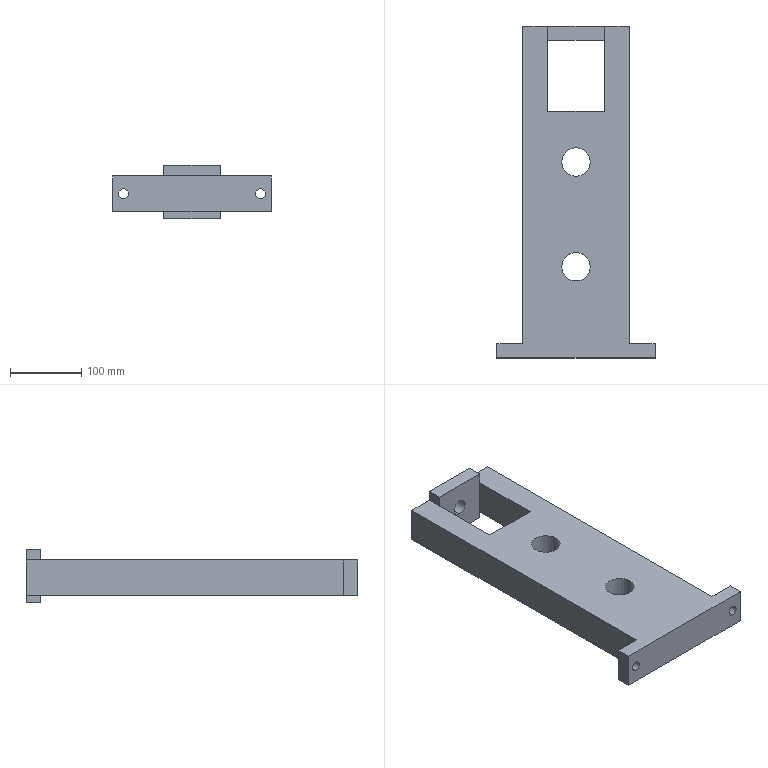Part | SolidWorks | features BaseBody 2 | 2 solids | 30 faces | box 222 x 466.001 x 75 mm | volume 3067581 mm3 | plane 20 | cylinder 10 | commonest cylinder face diameters 14 x4 40 x4 22 x2
STEP:
#1=CARTESIAN_POINT('',(0.,436.001,-8.5));
#2=VERTEX_POINT('',#1);
#3=CARTESIAN_POINT('',(0.,436.001,13.5));
#4=VERTEX_POINT('',#3);
#5=CARTESIAN_POINT('',(0.,436.001,2.5));
#6=DIRECTION('',(0.,1.,0.));
#7=DIRECTION('',(0.,0.,1.));
#8=AXIS2_PLACEMENT_3D('',#5,#6,#7);
#9=CIRCLE('',#8,11.);
#10=EDGE_CURVE('',#2,#4,#9,.T.);
#11=ORIENTED_EDGE('',*,*,#10,.F.);
#12=CARTESIAN_POINT('',(0.,456.001,-8.5));
#13=VERTEX_POINT('',#12);
#14=CARTESIAN_POINT('',(0.,456.001,-8.5));
#15=DIRECTION('',(0.,1.,0.));
#16=VECTOR('',#15,1000.);
#17=LINE('',#14,#16);
#18=EDGE_CURVE('',#2,#13,#17,.T.);
#19=ORIENTED_EDGE('',*,*,#18,.T.);
#20=CARTESIAN_POINT('',(0.,456.001,13.5));
#21=VERTEX_POINT('',#20);
#22=CARTESIAN_POINT('',(0.,456.001,2.5));
#23=DIRECTION('',(0.,1.,0.));
#24=DIRECTION('',(0.,0.,1.));
#25=AXIS2_PLACEMENT_3D('',#22,#23,#24);
#26=CIRCLE('',#25,11.);
#27=EDGE_CURVE('',#13,#21,#26,.T.);
#28=ORIENTED_EDGE('',*,*,#27,.T.);
#29=CARTESIAN_POINT('',(0.,456.001,13.5));
#30=DIRECTION('',(0.,1.,0.));
#31=VECTOR('',#30,1000.);
#32=LINE('',#29,#31);
#33=EDGE_CURVE('',#4,#21,#32,.T.);
#34=ORIENTED_EDGE('',*,*,#33,.F.);
#35=EDGE_LOOP('',(#11,#19,#28,#34));
#36=FACE_OUTER_BOUND('',#35,.T.);
#37=CARTESIAN_POINT('',(0.,456.001,2.5));
#38=DIRECTION('',(0.,1.,0.));
#39=DIRECTION('',(0.,0.,1.));
#40=AXIS2_PLACEMENT_3D('',#37,#38,#39);
#41=CYLINDRICAL_SURFACE('',#40,11.);
#42=ADVANCED_FACE('',(#36),#41,.F.);
#43=CARTESIAN_POINT('',(-40.,456.001,-35.));
#44=VERTEX_POINT('',#43);
#45=CARTESIAN_POINT('',(-40.,436.001,-35.));
#46=VERTEX_POINT('',#45);
#47=CARTESIAN_POINT('',(-40.,456.001,-35.));
#48=DIRECTION('',(0.,-1.,0.));
#49=VECTOR('',#48,1000.);
#50=LINE('',#47,#49);
#51=EDGE_CURVE('',#44,#46,#50,.T.);
#52=ORIENTED_EDGE('',*,*,#51,.F.);
#53=CARTESIAN_POINT('',(40.,456.001,-35.));
#54=VERTEX_POINT('',#53);
#55=CARTESIAN_POINT('',(-40.,456.001,-35.));
#56=DIRECTION('',(-1.,0.,0.));
#57=VECTOR('',#56,1000.);
#58=LINE('',#55,#57);
#59=EDGE_CURVE('',#54,#44,#58,.T.);
#60=ORIENTED_EDGE('',*,*,#59,.F.);
#61=CARTESIAN_POINT('',(40.,436.001,-35.));
#62=VERTEX_POINT('',#61);
#63=CARTESIAN_POINT('',(40.,456.001,-35.));
#64=DIRECTION('',(0.,1.,0.));
#65=VECTOR('',#64,1000.);
#66=LINE('',#63,#65);
#67=EDGE_CURVE('',#62,#54,#66,.T.);
#68=ORIENTED_EDGE('',*,*,#67,.F.);
#69=CARTESIAN_POINT('',(-40.,436.001,-35.));
#70=DIRECTION('',(1.,0.,0.));
#71=VECTOR('',#70,1000.);
#72=LINE('',#69,#71);
#73=EDGE_CURVE('',#46,#62,#72,.T.);
#74=ORIENTED_EDGE('',*,*,#73,.F.);
#75=EDGE_LOOP('',(#52,#60,#68,#74));
#76=FACE_OUTER_BOUND('',#75,.T.);
#77=CARTESIAN_POINT('',(0.,0.,-35.));
#78=DIRECTION('',(0.,0.,1.));
#79=DIRECTION('',(1.,0.,0.));
#80=AXIS2_PLACEMENT_3D('',#77,#78,#79);
#81=PLANE('',#80);
#82=ADVANCED_FACE('',(#76),#81,.F.);
#83=CARTESIAN_POINT('',(-40.,456.001,40.));
#84=VERTEX_POINT('',#83);
#85=CARTESIAN_POINT('',(-40.,436.001,40.));
#86=VERTEX_POINT('',#85);
#87=CARTESIAN_POINT('',(-40.,456.001,40.));
#88=DIRECTION('',(0.,-1.,0.));
#89=VECTOR('',#88,1000.);
#90=LINE('',#87,#89);
#91=EDGE_CURVE('',#84,#86,#90,.T.);
#92=ORIENTED_EDGE('',*,*,#91,.T.);
#93=CARTESIAN_POINT('',(40.,436.001,40.));
#94=VERTEX_POINT('',#93);
#95=CARTESIAN_POINT('',(-40.,436.001,40.));
#96=DIRECTION('',(1.,0.,0.));
#97=VECTOR('',#96,1000.);
#98=LINE('',#95,#97);
#99=EDGE_CURVE('',#86,#94,#98,.T.);
#100=ORIENTED_EDGE('',*,*,#99,.T.);
#101=CARTESIAN_POINT('',(40.,456.001,40.));
#102=VERTEX_POINT('',#101);
#103=CARTESIAN_POINT('',(40.,456.001,40.));
#104=DIRECTION('',(0.,1.,0.));
#105=VECTOR('',#104,1000.);
#106=LINE('',#103,#105);
#107=EDGE_CURVE('',#94,#102,#106,.T.);
#108=ORIENTED_EDGE('',*,*,#107,.T.);
#109=CARTESIAN_POINT('',(-40.,456.001,40.));
#110=DIRECTION('',(-1.,0.,0.));
#111=VECTOR('',#110,1000.);
#112=LINE('',#109,#111);
#113=EDGE_CURVE('',#102,#84,#112,.T.);
#114=ORIENTED_EDGE('',*,*,#113,.T.);
#115=EDGE_LOOP('',(#92,#100,#108,#114));
#116=FACE_OUTER_BOUND('',#115,.T.);
#117=CARTESIAN_POINT('',(0.,0.,40.));
#118=DIRECTION('',(0.,0.,1.));
#119=DIRECTION('',(1.,0.,0.));
#120=AXIS2_PLACEMENT_3D('',#117,#118,#119);
#121=PLANE('',#120);
#122=ADVANCED_FACE('',(#116),#121,.T.);
#123=CARTESIAN_POINT('',(0.,456.001,2.5));
#124=DIRECTION('',(0.,1.,0.));
#125=DIRECTION('',(0.,0.,1.));
#126=AXIS2_PLACEMENT_3D('',#123,#124,#125);
#127=CIRCLE('',#126,11.);
#128=EDGE_CURVE('',#21,#13,#127,.T.);
#129=ORIENTED_EDGE('',*,*,#128,.F.);
#130=ORIENTED_EDGE('',*,*,#27,.F.);
#131=EDGE_LOOP('',(#129,#130));
#132=FACE_BOUND('',#131,.T.);
#133=ORIENTED_EDGE('',*,*,#59,.T.);
#134=CARTESIAN_POINT('',(-40.,456.001,40.));
#135=DIRECTION('',(0.,0.,-1.));
#136=VECTOR('',#135,1000.);
#137=LINE('',#134,#136);
#138=EDGE_CURVE('',#84,#44,#137,.T.);
#139=ORIENTED_EDGE('',*,*,#138,.F.);
#140=ORIENTED_EDGE('',*,*,#113,.F.);
#141=CARTESIAN_POINT('',(40.,456.001,40.));
#142=DIRECTION('',(0.,0.,-1.));
#143=VECTOR('',#142,1000.);
#144=LINE('',#141,#143);
#145=EDGE_CURVE('',#102,#54,#144,.T.);
#146=ORIENTED_EDGE('',*,*,#145,.T.);
#147=EDGE_LOOP('',(#133,#139,#140,#146));
#148=FACE_OUTER_BOUND('',#147,.T.);
#149=CARTESIAN_POINT('',(-40.,456.001,40.));
#150=DIRECTION('',(0.,-1.,0.));
#151=DIRECTION('',(0.,0.,-1.));
#152=AXIS2_PLACEMENT_3D('',#149,#150,#151);
#153=PLANE('',#152);
#154=ADVANCED_FACE('',(#132,#148),#153,.F.);
#155=ORIENTED_EDGE('',*,*,#67,.T.);
#156=ORIENTED_EDGE('',*,*,#145,.F.);
#157=ORIENTED_EDGE('',*,*,#107,.F.);
#158=CARTESIAN_POINT('',(40.,436.001,40.));
#159=DIRECTION('',(0.,0.,-1.));
#160=VECTOR('',#159,1000.);
#161=LINE('',#158,#160);
#162=EDGE_CURVE('',#94,#62,#161,.T.);
#163=ORIENTED_EDGE('',*,*,#162,.T.);
#164=EDGE_LOOP('',(#155,#156,#157,#163));
#165=FACE_OUTER_BOUND('',#164,.T.);
#166=CARTESIAN_POINT('',(40.,456.001,40.));
#167=DIRECTION('',(-1.,0.,0.));
#168=DIRECTION('',(0.,0.,1.));
#169=AXIS2_PLACEMENT_3D('',#166,#167,#168);
#170=PLANE('',#169);
#171=ADVANCED_FACE('',(#165),#170,.F.);
#172=CARTESIAN_POINT('',(0.,436.001,2.5));
#173=DIRECTION('',(0.,1.,0.));
#174=DIRECTION('',(0.,0.,1.));
#175=AXIS2_PLACEMENT_3D('',#172,#173,#174);
#176=CIRCLE('',#175,11.);
#177=EDGE_CURVE('',#4,#2,#176,.T.);
#178=ORIENTED_EDGE('',*,*,#177,.T.);
#179=ORIENTED_EDGE('',*,*,#10,.T.);
#180=EDGE_LOOP('',(#178,#179));
#181=FACE_BOUND('',#180,.T.);
#182=ORIENTED_EDGE('',*,*,#73,.T.);
#183=ORIENTED_EDGE('',*,*,#162,.F.);
#184=ORIENTED_EDGE('',*,*,#99,.F.);
#185=CARTESIAN_POINT('',(-40.,436.001,40.));
#186=DIRECTION('',(0.,0.,-1.));
#187=VECTOR('',#186,1000.);
#188=LINE('',#185,#187);
#189=EDGE_CURVE('',#86,#46,#188,.T.);
#190=ORIENTED_EDGE('',*,*,#189,.T.);
#191=EDGE_LOOP('',(#182,#183,#184,#190));
#192=FACE_OUTER_BOUND('',#191,.T.);
#193=CARTESIAN_POINT('',(-40.,436.001,40.));
#194=DIRECTION('',(0.,1.,0.));
#195=DIRECTION('',(1.,0.,0.));
#196=AXIS2_PLACEMENT_3D('',#193,#194,#195);
#197=PLANE('',#196);
#198=ADVANCED_FACE('',(#181,#192),#197,.F.);
#199=ORIENTED_EDGE('',*,*,#51,.T.);
#200=ORIENTED_EDGE('',*,*,#189,.F.);
#201=ORIENTED_EDGE('',*,*,#91,.F.);
#202=ORIENTED_EDGE('',*,*,#138,.T.);
#203=EDGE_LOOP('',(#199,#200,#201,#202));
#204=FACE_OUTER_BOUND('',#203,.T.);
#205=CARTESIAN_POINT('',(-40.,456.001,40.));
#206=DIRECTION('',(1.,0.,0.));
#207=DIRECTION('',(0.,1.,0.));
#208=AXIS2_PLACEMENT_3D('',#205,#206,#207);
#209=PLANE('',#208);
#210=ADVANCED_FACE('',(#204),#209,.F.);
#211=ORIENTED_EDGE('',*,*,#18,.F.);
#212=ORIENTED_EDGE('',*,*,#177,.F.);
#213=ORIENTED_EDGE('',*,*,#33,.T.);
#214=ORIENTED_EDGE('',*,*,#128,.T.);
#215=EDGE_LOOP('',(#211,#212,#213,#214));
#216=FACE_OUTER_BOUND('',#215,.T.);
#217=CARTESIAN_POINT('',(0.,456.001,2.5));
#218=DIRECTION('',(0.,1.,0.));
#219=DIRECTION('',(0.,0.,1.));
#220=AXIS2_PLACEMENT_3D('',#217,#218,#219);
#221=CYLINDRICAL_SURFACE('',#220,11.);
#222=ADVANCED_FACE('',(#216),#221,.F.);
#223=CLOSED_SHELL('',(#42,#82,#122,#154,#171,#198,#210,#222));
#224=MANIFOLD_SOLID_BREP('',#223);
#225=CARTESIAN_POINT('',(-96.,-10.,-7.));
#226=VERTEX_POINT('',#225);
#227=CARTESIAN_POINT('',(-96.,-10.,7.));
#228=VERTEX_POINT('',#227);
#229=CARTESIAN_POINT('',(-96.,-10.,0.));
#230=DIRECTION('',(0.,1.,0.));
#231=DIRECTION('',(-1.,0.,0.));
#232=AXIS2_PLACEMENT_3D('',#229,#230,#231);
#233=CIRCLE('',#232,7.);
#234=EDGE_CURVE('',#226,#228,#233,.T.);
#235=ORIENTED_EDGE('',*,*,#234,.F.);
#236=CARTESIAN_POINT('',(-96.,10.,-7.));
#237=VERTEX_POINT('',#236);
#238=CARTESIAN_POINT('',(-96.,10.,-7.));
#239=DIRECTION('',(0.,1.,0.));
#240=VECTOR('',#239,1000.);
#241=LINE('',#238,#240);
#242=EDGE_CURVE('',#226,#237,#241,.T.);
#243=ORIENTED_EDGE('',*,*,#242,.T.);
#244=CARTESIAN_POINT('',(-96.,10.,7.));
#245=VERTEX_POINT('',#244);
#246=CARTESIAN_POINT('',(-96.,10.,0.));
#247=DIRECTION('',(0.,1.,0.));
#248=DIRECTION('',(1.,0.,0.));
#249=AXIS2_PLACEMENT_3D('',#246,#247,#248);
#250=CIRCLE('',#249,7.);
#251=EDGE_CURVE('',#237,#245,#250,.T.);
#252=ORIENTED_EDGE('',*,*,#251,.T.);
#253=CARTESIAN_POINT('',(-96.,10.,7.));
#254=DIRECTION('',(0.,1.,0.));
#255=VECTOR('',#254,1000.);
#256=LINE('',#253,#255);
#257=EDGE_CURVE('',#228,#245,#256,.T.);
#258=ORIENTED_EDGE('',*,*,#257,.F.);
#259=EDGE_LOOP('',(#235,#243,#252,#258));
#260=FACE_OUTER_BOUND('',#259,.T.);
#261=CARTESIAN_POINT('',(-96.,10.,0.));
#262=DIRECTION('',(0.,1.,0.));
#263=DIRECTION('',(0.,0.,1.));
#264=AXIS2_PLACEMENT_3D('',#261,#262,#263);
#265=CYLINDRICAL_SURFACE('',#264,7.);
#266=ADVANCED_FACE('',(#260),#265,.F.);
#267=CARTESIAN_POINT('',(96.,-10.,-7.));
#268=VERTEX_POINT('',#267);
#269=CARTESIAN_POINT('',(96.,-10.,7.));
#270=VERTEX_POINT('',#269);
#271=CARTESIAN_POINT('',(96.,-10.,0.));
#272=DIRECTION('',(0.,1.,0.));
#273=DIRECTION('',(-1.,0.,0.));
#274=AXIS2_PLACEMENT_3D('',#271,#272,#273);
#275=CIRCLE('',#274,7.);
#276=EDGE_CURVE('',#268,#270,#275,.T.);
#277=ORIENTED_EDGE('',*,*,#276,.F.);
#278=CARTESIAN_POINT('',(96.,10.,-7.));
#279=VERTEX_POINT('',#278);
#280=CARTESIAN_POINT('',(96.,10.,-7.));
#281=DIRECTION('',(0.,1.,0.));
#282=VECTOR('',#281,1000.);
#283=LINE('',#280,#282);
#284=EDGE_CURVE('',#268,#279,#283,.T.);
#285=ORIENTED_EDGE('',*,*,#284,.T.);
#286=CARTESIAN_POINT('',(96.,10.,7.));
#287=VERTEX_POINT('',#286);
#288=CARTESIAN_POINT('',(96.,10.,0.));
#289=DIRECTION('',(0.,1.,0.));
#290=DIRECTION('',(1.,0.,0.));
#291=AXIS2_PLACEMENT_3D('',#288,#289,#290);
#292=CIRCLE('',#291,7.);
#293=EDGE_CURVE('',#279,#287,#292,.T.);
#294=ORIENTED_EDGE('',*,*,#293,.T.);
#295=CARTESIAN_POINT('',(96.,10.,7.));
#296=DIRECTION('',(0.,1.,0.));
#297=VECTOR('',#296,1000.);
#298=LINE('',#295,#297);
#299=EDGE_CURVE('',#270,#287,#298,.T.);
#300=ORIENTED_EDGE('',*,*,#299,.F.);
#301=EDGE_LOOP('',(#277,#285,#294,#300));
#302=FACE_OUTER_BOUND('',#301,.T.);
#303=CARTESIAN_POINT('',(96.,10.,0.));
#304=DIRECTION('',(0.,1.,0.));
#305=DIRECTION('',(0.,0.,1.));
#306=AXIS2_PLACEMENT_3D('',#303,#304,#305);
#307=CYLINDRICAL_SURFACE('',#306,7.);
#308=ADVANCED_FACE('',(#302),#307,.F.);
#309=CARTESIAN_POINT('',(-20.,265.,25.));
#310=VERTEX_POINT('',#309);
#311=CARTESIAN_POINT('',(20.,265.,25.));
#312=VERTEX_POINT('',#311);
#313=CARTESIAN_POINT('',(0.,265.,25.));
#314=DIRECTION('',(0.,0.,1.));
#315=DIRECTION('',(1.,0.,0.));
#316=AXIS2_PLACEMENT_3D('',#313,#314,#315);
#317=CIRCLE('',#316,20.);
#318=EDGE_CURVE('',#310,#312,#317,.T.);
#319=ORIENTED_EDGE('',*,*,#318,.T.);
#320=CARTESIAN_POINT('',(20.,265.,-25.));
#321=VERTEX_POINT('',#320);
#322=CARTESIAN_POINT('',(20.,265.,20.));
#323=DIRECTION('',(0.,0.,-1.));
#324=VECTOR('',#323,1000.);
#325=LINE('',#322,#324);
#326=EDGE_CURVE('',#312,#321,#325,.T.);
#327=ORIENTED_EDGE('',*,*,#326,.T.);
#328=CARTESIAN_POINT('',(-20.,265.,-25.));
#329=VERTEX_POINT('',#328);
#330=CARTESIAN_POINT('',(0.,265.,-25.));
#331=DIRECTION('',(0.,0.,1.));
#332=DIRECTION('',(1.,0.,0.));
#333=AXIS2_PLACEMENT_3D('',#330,#331,#332);
#334=CIRCLE('',#333,20.);
#335=EDGE_CURVE('',#329,#321,#334,.T.);
#336=ORIENTED_EDGE('',*,*,#335,.F.);
#337=CARTESIAN_POINT('',(-20.,265.,20.));
#338=DIRECTION('',(0.,0.,-1.));
#339=VECTOR('',#338,1000.);
#340=LINE('',#337,#339);
#341=EDGE_CURVE('',#310,#329,#340,.T.);
#342=ORIENTED_EDGE('',*,*,#341,.F.);
#343=EDGE_LOOP('',(#319,#327,#336,#342));
#344=FACE_OUTER_BOUND('',#343,.T.);
#345=CARTESIAN_POINT('',(0.,265.,20.));
#346=DIRECTION('',(0.,0.,-1.));
#347=DIRECTION('',(-1.,0.,0.));
#348=AXIS2_PLACEMENT_3D('',#345,#346,#347);
#349=CYLINDRICAL_SURFACE('',#348,20.);
#350=ADVANCED_FACE('',(#344),#349,.F.);
#351=CARTESIAN_POINT('',(-20.,118.,25.));
#352=VERTEX_POINT('',#351);
#353=CARTESIAN_POINT('',(20.,118.,25.));
#354=VERTEX_POINT('',#353);
#355=CARTESIAN_POINT('',(0.,118.,25.));
#356=DIRECTION('',(0.,0.,1.));
#357=DIRECTION('',(1.,0.,0.));
#358=AXIS2_PLACEMENT_3D('',#355,#356,#357);
#359=CIRCLE('',#358,20.);
#360=EDGE_CURVE('',#352,#354,#359,.T.);
#361=ORIENTED_EDGE('',*,*,#360,.T.);
#362=CARTESIAN_POINT('',(20.,118.,-25.));
#363=VERTEX_POINT('',#362);
#364=CARTESIAN_POINT('',(20.,118.,20.));
#365=DIRECTION('',(0.,0.,-1.));
#366=VECTOR('',#365,1000.);
#367=LINE('',#364,#366);
#368=EDGE_CURVE('',#354,#363,#367,.T.);
#369=ORIENTED_EDGE('',*,*,#368,.T.);
#370=CARTESIAN_POINT('',(-20.,118.,-25.));
#371=VERTEX_POINT('',#370);
#372=CARTESIAN_POINT('',(0.,118.,-25.));
#373=DIRECTION('',(0.,0.,1.));
#374=DIRECTION('',(1.,0.,0.));
#375=AXIS2_PLACEMENT_3D('',#372,#373,#374);
#376=CIRCLE('',#375,20.);
#377=EDGE_CURVE('',#371,#363,#376,.T.);
#378=ORIENTED_EDGE('',*,*,#377,.F.);
#379=CARTESIAN_POINT('',(-20.,118.,20.));
#380=DIRECTION('',(0.,0.,-1.));
#381=VECTOR('',#380,1000.);
#382=LINE('',#379,#381);
#383=EDGE_CURVE('',#352,#371,#382,.T.);
#384=ORIENTED_EDGE('',*,*,#383,.F.);
#385=EDGE_LOOP('',(#361,#369,#378,#384));
#386=FACE_OUTER_BOUND('',#385,.T.);
#387=CARTESIAN_POINT('',(0.,118.,20.));
#388=DIRECTION('',(0.,0.,-1.));
#389=DIRECTION('',(-1.,0.,0.));
#390=AXIS2_PLACEMENT_3D('',#387,#388,#389);
#391=CYLINDRICAL_SURFACE('',#390,20.);
#392=ADVANCED_FACE('',(#386),#391,.F.);
#393=CARTESIAN_POINT('',(40.,336.001,-25.));
#394=VERTEX_POINT('',#393);
#395=CARTESIAN_POINT('',(-40.,336.001,-25.));
#396=VERTEX_POINT('',#395);
#397=CARTESIAN_POINT('',(-40.,336.001,-25.));
#398=DIRECTION('',(-1.,0.,0.));
#399=VECTOR('',#398,1000.);
#400=LINE('',#397,#399);
#401=EDGE_CURVE('',#394,#396,#400,.T.);
#402=ORIENTED_EDGE('',*,*,#401,.T.);
#403=CARTESIAN_POINT('',(-40.,336.001,25.));
#404=VERTEX_POINT('',#403);
#405=CARTESIAN_POINT('',(-40.,336.001,-25.001));
#406=DIRECTION('',(0.,0.,1.));
#407=VECTOR('',#406,1000.);
#408=LINE('',#405,#407);
#409=EDGE_CURVE('',#396,#404,#408,.T.);
#410=ORIENTED_EDGE('',*,*,#409,.T.);
#411=CARTESIAN_POINT('',(40.,336.001,25.));
#412=VERTEX_POINT('',#411);
#413=CARTESIAN_POINT('',(0.,336.001,25.));
#414=DIRECTION('',(1.,0.,0.));
#415=VECTOR('',#414,1000.);
#416=LINE('',#413,#415);
#417=EDGE_CURVE('',#404,#412,#416,.T.);
#418=ORIENTED_EDGE('',*,*,#417,.T.);
#419=CARTESIAN_POINT('',(40.,336.001,-25.001));
#420=DIRECTION('',(0.,0.,1.));
#421=VECTOR('',#420,1000.);
#422=LINE('',#419,#421);
#423=EDGE_CURVE('',#394,#412,#422,.T.);
#424=ORIENTED_EDGE('',*,*,#423,.F.);
#425=EDGE_LOOP('',(#402,#410,#418,#424));
#426=FACE_OUTER_BOUND('',#425,.T.);
#427=CARTESIAN_POINT('',(-40.,336.001,-25.001));
#428=DIRECTION('',(0.,-1.,0.));
#429=DIRECTION('',(0.,0.,-1.));
#430=AXIS2_PLACEMENT_3D('',#427,#428,#429);
#431=PLANE('',#430);
#432=ADVANCED_FACE('',(#426),#431,.F.);
#433=CARTESIAN_POINT('',(40.,456.001,-25.));
#434=VERTEX_POINT('',#433);
#435=CARTESIAN_POINT('',(40.,456.001,-25.));
#436=DIRECTION('',(0.,-1.,0.));
#437=VECTOR('',#436,1000.);
#438=LINE('',#435,#437);
#439=EDGE_CURVE('',#434,#394,#438,.T.);
#440=ORIENTED_EDGE('',*,*,#439,.T.);
#441=ORIENTED_EDGE('',*,*,#423,.T.);
#442=CARTESIAN_POINT('',(40.,456.001,25.));
#443=VERTEX_POINT('',#442);
#444=CARTESIAN_POINT('',(40.,456.001,25.));
#445=DIRECTION('',(0.,1.,0.));
#446=VECTOR('',#445,1000.);
#447=LINE('',#444,#446);
#448=EDGE_CURVE('',#412,#443,#447,.T.);
#449=ORIENTED_EDGE('',*,*,#448,.T.);
#450=CARTESIAN_POINT('',(40.,456.001,-25.001));
#451=DIRECTION('',(0.,0.,1.));
#452=VECTOR('',#451,1000.);
#453=LINE('',#450,#452);
#454=EDGE_CURVE('',#434,#443,#453,.T.);
#455=ORIENTED_EDGE('',*,*,#454,.F.);
#456=EDGE_LOOP('',(#440,#441,#449,#455));
#457=FACE_OUTER_BOUND('',#456,.T.);
#458=CARTESIAN_POINT('',(40.,456.001,-25.001));
#459=DIRECTION('',(1.,0.,0.));
#460=DIRECTION('',(0.,1.,0.));
#461=AXIS2_PLACEMENT_3D('',#458,#459,#460);
#462=PLANE('',#461);
#463=ADVANCED_FACE('',(#457),#462,.F.);
#464=CARTESIAN_POINT('',(-40.,456.001,-25.));
#465=VERTEX_POINT('',#464);
#466=CARTESIAN_POINT('',(-40.,456.001,-25.));
#467=DIRECTION('',(0.,1.,0.));
#468=VECTOR('',#467,1000.);
#469=LINE('',#466,#468);
#470=EDGE_CURVE('',#396,#465,#469,.T.);
#471=ORIENTED_EDGE('',*,*,#470,.T.);
#472=CARTESIAN_POINT('',(-40.,456.001,25.));
#473=VERTEX_POINT('',#472);
#474=CARTESIAN_POINT('',(-40.,456.001,-25.001));
#475=DIRECTION('',(0.,0.,1.));
#476=VECTOR('',#475,1000.);
#477=LINE('',#474,#476);
#478=EDGE_CURVE('',#465,#473,#477,.T.);
#479=ORIENTED_EDGE('',*,*,#478,.T.);
#480=CARTESIAN_POINT('',(-40.,456.001,25.));
#481=DIRECTION('',(0.,-1.,0.));
#482=VECTOR('',#481,1000.);
#483=LINE('',#480,#482);
#484=EDGE_CURVE('',#473,#404,#483,.T.);
#485=ORIENTED_EDGE('',*,*,#484,.T.);
#486=ORIENTED_EDGE('',*,*,#409,.F.);
#487=EDGE_LOOP('',(#471,#479,#485,#486));
#488=FACE_OUTER_BOUND('',#487,.T.);
#489=CARTESIAN_POINT('',(-40.,456.001,-25.001));
#490=DIRECTION('',(-1.,0.,0.));
#491=DIRECTION('',(0.,0.,1.));
#492=AXIS2_PLACEMENT_3D('',#489,#490,#491);
#493=PLANE('',#492);
#494=ADVANCED_FACE('',(#488),#493,.F.);
#495=CARTESIAN_POINT('',(96.,-10.,0.));
#496=DIRECTION('',(0.,1.,0.));
#497=DIRECTION('',(-1.,0.,0.));
#498=AXIS2_PLACEMENT_3D('',#495,#496,#497);
#499=CIRCLE('',#498,7.);
#500=EDGE_CURVE('',#270,#268,#499,.T.);
#501=ORIENTED_EDGE('',*,*,#500,.T.);
#502=ORIENTED_EDGE('',*,*,#276,.T.);
#503=EDGE_LOOP('',(#501,#502));
#504=FACE_BOUND('',#503,.T.);
#505=CARTESIAN_POINT('',(-96.,-10.,0.));
#506=DIRECTION('',(0.,1.,0.));
#507=DIRECTION('',(-1.,0.,0.));
#508=AXIS2_PLACEMENT_3D('',#505,#506,#507);
#509=CIRCLE('',#508,7.);
#510=EDGE_CURVE('',#228,#226,#509,.T.);
#511=ORIENTED_EDGE('',*,*,#510,.T.);
#512=ORIENTED_EDGE('',*,*,#234,.T.);
#513=EDGE_LOOP('',(#511,#512));
#514=FACE_BOUND('',#513,.T.);
#515=CARTESIAN_POINT('',(-111.,-10.,-25.));
#516=VERTEX_POINT('',#515);
#517=CARTESIAN_POINT('',(111.,-10.,-25.));
#518=VERTEX_POINT('',#517);
#519=CARTESIAN_POINT('',(-88.,-10.,-25.));
#520=DIRECTION('',(1.,0.,0.));
#521=VECTOR('',#520,1000.);
#522=LINE('',#519,#521);
#523=EDGE_CURVE('',#516,#518,#522,.T.);
#524=ORIENTED_EDGE('',*,*,#523,.T.);
#525=CARTESIAN_POINT('',(111.,-10.,25.));
#526=VERTEX_POINT('',#525);
#527=CARTESIAN_POINT('',(111.,-10.,20.));
#528=DIRECTION('',(0.,0.,-1.));
#529=VECTOR('',#528,1000.);
#530=LINE('',#527,#529);
#531=EDGE_CURVE('',#526,#518,#530,.T.);
#532=ORIENTED_EDGE('',*,*,#531,.F.);
#533=CARTESIAN_POINT('',(-111.,-10.,25.));
#534=VERTEX_POINT('',#533);
#535=CARTESIAN_POINT('',(-88.,-10.,25.));
#536=DIRECTION('',(1.,0.,0.));
#537=VECTOR('',#536,1000.);
#538=LINE('',#535,#537);
#539=EDGE_CURVE('',#534,#526,#538,.T.);
#540=ORIENTED_EDGE('',*,*,#539,.F.);
#541=CARTESIAN_POINT('',(-111.,-10.,20.));
#542=DIRECTION('',(0.,0.,-1.));
#543=VECTOR('',#542,1000.);
#544=LINE('',#541,#543);
#545=EDGE_CURVE('',#534,#516,#544,.T.);
#546=ORIENTED_EDGE('',*,*,#545,.T.);
#547=EDGE_LOOP('',(#524,#532,#540,#546));
#548=FACE_OUTER_BOUND('',#547,.T.);
#549=CARTESIAN_POINT('',(-88.,-10.,20.));
#550=DIRECTION('',(0.,1.,0.));
#551=DIRECTION('',(1.,0.,0.));
#552=AXIS2_PLACEMENT_3D('',#549,#550,#551);
#553=PLANE('',#552);
#554=ADVANCED_FACE('',(#504,#514,#548),#553,.F.);
#555=CARTESIAN_POINT('',(-111.,10.,-25.));
#556=VERTEX_POINT('',#555);
#557=CARTESIAN_POINT('',(-111.,10.,-25.));
#558=DIRECTION('',(0.,-1.,0.));
#559=VECTOR('',#558,1000.);
#560=LINE('',#557,#559);
#561=EDGE_CURVE('',#556,#516,#560,.T.);
#562=ORIENTED_EDGE('',*,*,#561,.T.);
#563=ORIENTED_EDGE('',*,*,#545,.F.);
#564=CARTESIAN_POINT('',(-111.,10.,25.));
#565=VERTEX_POINT('',#564);
#566=CARTESIAN_POINT('',(-111.,10.,25.));
#567=DIRECTION('',(0.,-1.,0.));
#568=VECTOR('',#567,1000.);
#569=LINE('',#566,#568);
#570=EDGE_CURVE('',#565,#534,#569,.T.);
#571=ORIENTED_EDGE('',*,*,#570,.F.);
#572=CARTESIAN_POINT('',(-111.,10.,20.));
#573=DIRECTION('',(0.,0.,-1.));
#574=VECTOR('',#573,1000.);
#575=LINE('',#572,#574);
#576=EDGE_CURVE('',#565,#556,#575,.T.);
#577=ORIENTED_EDGE('',*,*,#576,.T.);
#578=EDGE_LOOP('',(#562,#563,#571,#577));
#579=FACE_OUTER_BOUND('',#578,.T.);
#580=CARTESIAN_POINT('',(-111.,10.,20.));
#581=DIRECTION('',(1.,0.,0.));
#582=DIRECTION('',(0.,1.,0.));
#583=AXIS2_PLACEMENT_3D('',#580,#581,#582);
#584=PLANE('',#583);
#585=ADVANCED_FACE('',(#579),#584,.F.);
#586=CARTESIAN_POINT('',(-96.,10.,0.));
#587=DIRECTION('',(0.,1.,0.));
#588=DIRECTION('',(1.,0.,0.));
#589=AXIS2_PLACEMENT_3D('',#586,#587,#588);
#590=CIRCLE('',#589,7.);
#591=EDGE_CURVE('',#245,#237,#590,.T.);
#592=ORIENTED_EDGE('',*,*,#591,.F.);
#593=ORIENTED_EDGE('',*,*,#251,.F.);
#594=EDGE_LOOP('',(#592,#593));
#595=FACE_BOUND('',#594,.T.);
#596=CARTESIAN_POINT('',(-75.,10.,-25.));
#597=VERTEX_POINT('',#596);
#598=CARTESIAN_POINT('',(-88.,10.,-25.));
#599=DIRECTION('',(-1.,0.,0.));
#600=VECTOR('',#599,1000.);
#601=LINE('',#598,#600);
#602=EDGE_CURVE('',#597,#556,#601,.T.);
#603=ORIENTED_EDGE('',*,*,#602,.T.);
#604=ORIENTED_EDGE('',*,*,#576,.F.);
#605=CARTESIAN_POINT('',(-75.,10.,25.));
#606=VERTEX_POINT('',#605);
#607=CARTESIAN_POINT('',(-88.,10.,25.));
#608=DIRECTION('',(-1.,0.,0.));
#609=VECTOR('',#608,1000.);
#610=LINE('',#607,#609);
#611=EDGE_CURVE('',#606,#565,#610,.T.);
#612=ORIENTED_EDGE('',*,*,#611,.F.);
#613=CARTESIAN_POINT('',(-75.,10.,20.));
#614=DIRECTION('',(0.,0.,-1.));
#615=VECTOR('',#614,1000.);
#616=LINE('',#613,#615);
#617=EDGE_CURVE('',#606,#597,#616,.T.);
#618=ORIENTED_EDGE('',*,*,#617,.T.);
#619=EDGE_LOOP('',(#603,#604,#612,#618));
#620=FACE_OUTER_BOUND('',#619,.T.);
#621=CARTESIAN_POINT('',(-88.,10.,20.));
#622=DIRECTION('',(0.,-1.,0.));
#623=DIRECTION('',(0.,0.,-1.));
#624=AXIS2_PLACEMENT_3D('',#621,#622,#623);
#625=PLANE('',#624);
#626=ADVANCED_FACE('',(#595,#620),#625,.F.);
#627=CARTESIAN_POINT('',(-75.,456.001,-25.));
#628=VERTEX_POINT('',#627);
#629=CARTESIAN_POINT('',(-75.,460.,-25.));
#630=DIRECTION('',(0.,-1.,0.));
#631=VECTOR('',#630,1000.);
#632=LINE('',#629,#631);
#633=EDGE_CURVE('',#628,#597,#632,.T.);
#634=ORIENTED_EDGE('',*,*,#633,.T.);
#635=ORIENTED_EDGE('',*,*,#617,.F.);
#636=CARTESIAN_POINT('',(-75.,456.001,25.));
#637=VERTEX_POINT('',#636);
#638=CARTESIAN_POINT('',(-75.,460.,25.));
#639=DIRECTION('',(0.,-1.,0.));
#640=VECTOR('',#639,1000.);
#641=LINE('',#638,#640);
#642=EDGE_CURVE('',#637,#606,#641,.T.);
#643=ORIENTED_EDGE('',*,*,#642,.F.);
#644=CARTESIAN_POINT('',(-75.,456.001,20.));
#645=DIRECTION('',(0.,0.,-1.));
#646=VECTOR('',#645,1000.);
#647=LINE('',#644,#646);
#648=EDGE_CURVE('',#637,#628,#647,.T.);
#649=ORIENTED_EDGE('',*,*,#648,.T.);
#650=EDGE_LOOP('',(#634,#635,#643,#649));
#651=FACE_OUTER_BOUND('',#650,.T.);
#652=CARTESIAN_POINT('',(-75.,460.,20.));
#653=DIRECTION('',(1.,0.,0.));
#654=DIRECTION('',(0.,1.,0.));
#655=AXIS2_PLACEMENT_3D('',#652,#653,#654);
#656=PLANE('',#655);
#657=ADVANCED_FACE('',(#651),#656,.F.);
#658=CARTESIAN_POINT('',(75.,456.001,-25.));
#659=VERTEX_POINT('',#658);
#660=CARTESIAN_POINT('',(-40.,456.001,-25.));
#661=DIRECTION('',(-1.,0.,0.));
#662=VECTOR('',#661,1000.);
#663=LINE('',#660,#662);
#664=EDGE_CURVE('',#659,#434,#663,.T.);
#665=ORIENTED_EDGE('',*,*,#664,.T.);
#666=ORIENTED_EDGE('',*,*,#454,.T.);
#667=CARTESIAN_POINT('',(75.,456.001,25.));
#668=VERTEX_POINT('',#667);
#669=CARTESIAN_POINT('',(-40.,456.001,25.));
#670=DIRECTION('',(-1.,0.,0.));
#671=VECTOR('',#670,1000.);
#672=LINE('',#669,#671);
#673=EDGE_CURVE('',#668,#443,#672,.T.);
#674=ORIENTED_EDGE('',*,*,#673,.F.);
#675=CARTESIAN_POINT('',(75.,456.001,20.));
#676=DIRECTION('',(0.,0.,-1.));
#677=VECTOR('',#676,1000.);
#678=LINE('',#675,#677);
#679=EDGE_CURVE('',#668,#659,#678,.T.);
#680=ORIENTED_EDGE('',*,*,#679,.T.);
#681=EDGE_LOOP('',(#665,#666,#674,#680));
#682=FACE_OUTER_BOUND('',#681,.T.);
#683=CARTESIAN_POINT('',(-40.,456.001,20.));
#684=DIRECTION('',(0.,-1.,0.));
#685=DIRECTION('',(0.,0.,-1.));
#686=AXIS2_PLACEMENT_3D('',#683,#684,#685);
#687=PLANE('',#686);
#688=ADVANCED_FACE('',(#682),#687,.F.);
#689=CARTESIAN_POINT('',(75.,10.,-25.));
#690=VERTEX_POINT('',#689);
#691=CARTESIAN_POINT('',(75.,460.,-25.));
#692=DIRECTION('',(0.,1.,0.));
#693=VECTOR('',#692,1000.);
#694=LINE('',#691,#693);
#695=EDGE_CURVE('',#690,#659,#694,.T.);
#696=ORIENTED_EDGE('',*,*,#695,.T.);
#697=ORIENTED_EDGE('',*,*,#679,.F.);
#698=CARTESIAN_POINT('',(75.,10.,25.));
#699=VERTEX_POINT('',#698);
#700=CARTESIAN_POINT('',(75.,460.,25.));
#701=DIRECTION('',(0.,1.,0.));
#702=VECTOR('',#701,1000.);
#703=LINE('',#700,#702);
#704=EDGE_CURVE('',#699,#668,#703,.T.);
#705=ORIENTED_EDGE('',*,*,#704,.F.);
#706=CARTESIAN_POINT('',(75.,10.,20.));
#707=DIRECTION('',(0.,0.,-1.));
#708=VECTOR('',#707,1000.);
#709=LINE('',#706,#708);
#710=EDGE_CURVE('',#699,#690,#709,.T.);
#711=ORIENTED_EDGE('',*,*,#710,.T.);
#712=EDGE_LOOP('',(#696,#697,#705,#711));
#713=FACE_OUTER_BOUND('',#712,.T.);
#714=CARTESIAN_POINT('',(75.,460.,20.));
#715=DIRECTION('',(-1.,0.,0.));
#716=DIRECTION('',(0.,0.,1.));
#717=AXIS2_PLACEMENT_3D('',#714,#715,#716);
#718=PLANE('',#717);
#719=ADVANCED_FACE('',(#713),#718,.F.);
#720=CARTESIAN_POINT('',(96.,10.,0.));
#721=DIRECTION('',(0.,1.,0.));
#722=DIRECTION('',(1.,0.,0.));
#723=AXIS2_PLACEMENT_3D('',#720,#721,#722);
#724=CIRCLE('',#723,7.);
#725=EDGE_CURVE('',#287,#279,#724,.T.);
#726=ORIENTED_EDGE('',*,*,#725,.F.);
#727=ORIENTED_EDGE('',*,*,#293,.F.);
#728=EDGE_LOOP('',(#726,#727));
#729=FACE_BOUND('',#728,.T.);
#730=CARTESIAN_POINT('',(111.,10.,-25.));
#731=VERTEX_POINT('',#730);
#732=CARTESIAN_POINT('',(40.,10.,-25.));
#733=DIRECTION('',(-1.,0.,0.));
#734=VECTOR('',#733,1000.);
#735=LINE('',#732,#734);
#736=EDGE_CURVE('',#731,#690,#735,.T.);
#737=ORIENTED_EDGE('',*,*,#736,.T.);
#738=ORIENTED_EDGE('',*,*,#710,.F.);
#739=CARTESIAN_POINT('',(111.,10.,25.));
#740=VERTEX_POINT('',#739);
#741=CARTESIAN_POINT('',(40.,10.,25.));
#742=DIRECTION('',(-1.,0.,0.));
#743=VECTOR('',#742,1000.);
#744=LINE('',#741,#743);
#745=EDGE_CURVE('',#740,#699,#744,.T.);
#746=ORIENTED_EDGE('',*,*,#745,.F.);
#747=CARTESIAN_POINT('',(111.,10.,20.));
#748=DIRECTION('',(0.,0.,-1.));
#749=VECTOR('',#748,1000.);
#750=LINE('',#747,#749);
#751=EDGE_CURVE('',#740,#731,#750,.T.);
#752=ORIENTED_EDGE('',*,*,#751,.T.);
#753=EDGE_LOOP('',(#737,#738,#746,#752));
#754=FACE_OUTER_BOUND('',#753,.T.);
#755=CARTESIAN_POINT('',(40.,10.,20.));
#756=DIRECTION('',(0.,-1.,0.));
#757=DIRECTION('',(-1.,0.,0.));
#758=AXIS2_PLACEMENT_3D('',#755,#756,#757);
#759=PLANE('',#758);
#760=ADVANCED_FACE('',(#729,#754),#759,.F.);
#761=CARTESIAN_POINT('',(111.,10.,-25.));
#762=DIRECTION('',(0.,1.,0.));
#763=VECTOR('',#762,1000.);
#764=LINE('',#761,#763);
#765=EDGE_CURVE('',#518,#731,#764,.T.);
#766=ORIENTED_EDGE('',*,*,#765,.T.);
#767=ORIENTED_EDGE('',*,*,#751,.F.);
#768=CARTESIAN_POINT('',(111.,10.,25.));
#769=DIRECTION('',(0.,1.,0.));
#770=VECTOR('',#769,1000.);
#771=LINE('',#768,#770);
#772=EDGE_CURVE('',#526,#740,#771,.T.);
#773=ORIENTED_EDGE('',*,*,#772,.F.);
#774=ORIENTED_EDGE('',*,*,#531,.T.);
#775=EDGE_LOOP('',(#766,#767,#773,#774));
#776=FACE_OUTER_BOUND('',#775,.T.);
#777=CARTESIAN_POINT('',(111.,10.,20.));
#778=DIRECTION('',(-1.,0.,0.));
#779=DIRECTION('',(0.,0.,1.));
#780=AXIS2_PLACEMENT_3D('',#777,#778,#779);
#781=PLANE('',#780);
#782=ADVANCED_FACE('',(#776),#781,.F.);
#783=ORIENTED_EDGE('',*,*,#335,.T.);
#784=CARTESIAN_POINT('',(0.,265.,-25.));
#785=DIRECTION('',(0.,0.,1.));
#786=DIRECTION('',(1.,0.,0.));
#787=AXIS2_PLACEMENT_3D('',#784,#785,#786);
#788=CIRCLE('',#787,20.);
#789=EDGE_CURVE('',#321,#329,#788,.T.);
#790=ORIENTED_EDGE('',*,*,#789,.T.);
#791=EDGE_LOOP('',(#783,#790));
#792=FACE_BOUND('',#791,.T.);
#793=ORIENTED_EDGE('',*,*,#377,.T.);
#794=CARTESIAN_POINT('',(0.,118.,-25.));
#795=DIRECTION('',(0.,0.,1.));
#796=DIRECTION('',(1.,0.,0.));
#797=AXIS2_PLACEMENT_3D('',#794,#795,#796);
#798=CIRCLE('',#797,20.);
#799=EDGE_CURVE('',#363,#371,#798,.T.);
#800=ORIENTED_EDGE('',*,*,#799,.T.);
#801=EDGE_LOOP('',(#793,#800));
#802=FACE_BOUND('',#801,.T.);
#803=CARTESIAN_POINT('',(-40.,456.001,-25.));
#804=DIRECTION('',(-1.,0.,0.));
#805=VECTOR('',#804,1000.);
#806=LINE('',#803,#805);
#807=EDGE_CURVE('',#465,#628,#806,.T.);
#808=ORIENTED_EDGE('',*,*,#807,.F.);
#809=ORIENTED_EDGE('',*,*,#470,.F.);
#810=ORIENTED_EDGE('',*,*,#401,.F.);
#811=ORIENTED_EDGE('',*,*,#439,.F.);
#812=ORIENTED_EDGE('',*,*,#664,.F.);
#813=ORIENTED_EDGE('',*,*,#695,.F.);
#814=ORIENTED_EDGE('',*,*,#736,.F.);
#815=ORIENTED_EDGE('',*,*,#765,.F.);
#816=ORIENTED_EDGE('',*,*,#523,.F.);
#817=ORIENTED_EDGE('',*,*,#561,.F.);
#818=ORIENTED_EDGE('',*,*,#602,.F.);
#819=ORIENTED_EDGE('',*,*,#633,.F.);
#820=EDGE_LOOP('',(#808,#809,#810,#811,#812,#813,#814,#815,#816,#817,#818,#819));
#821=FACE_OUTER_BOUND('',#820,.T.);
#822=CARTESIAN_POINT('',(0.,0.,-25.));
#823=DIRECTION('',(0.,0.,1.));
#824=DIRECTION('',(1.,0.,0.));
#825=AXIS2_PLACEMENT_3D('',#822,#823,#824);
#826=PLANE('',#825);
#827=ADVANCED_FACE('',(#792,#802,#821),#826,.F.);
#828=ORIENTED_EDGE('',*,*,#318,.F.);
#829=CARTESIAN_POINT('',(0.,265.,25.));
#830=DIRECTION('',(0.,0.,1.));
#831=DIRECTION('',(1.,0.,0.));
#832=AXIS2_PLACEMENT_3D('',#829,#830,#831);
#833=CIRCLE('',#832,20.);
#834=EDGE_CURVE('',#312,#310,#833,.T.);
#835=ORIENTED_EDGE('',*,*,#834,.F.);
#836=EDGE_LOOP('',(#828,#835));
#837=FACE_BOUND('',#836,.T.);
#838=ORIENTED_EDGE('',*,*,#360,.F.);
#839=CARTESIAN_POINT('',(0.,118.,25.));
#840=DIRECTION('',(0.,0.,1.));
#841=DIRECTION('',(1.,0.,0.));
#842=AXIS2_PLACEMENT_3D('',#839,#840,#841);
#843=CIRCLE('',#842,20.);
#844=EDGE_CURVE('',#354,#352,#843,.T.);
#845=ORIENTED_EDGE('',*,*,#844,.F.);
#846=EDGE_LOOP('',(#838,#845));
#847=FACE_BOUND('',#846,.T.);
#848=ORIENTED_EDGE('',*,*,#484,.F.);
#849=CARTESIAN_POINT('',(-40.,456.001,25.));
#850=DIRECTION('',(-1.,0.,0.));
#851=VECTOR('',#850,1000.);
#852=LINE('',#849,#851);
#853=EDGE_CURVE('',#473,#637,#852,.T.);
#854=ORIENTED_EDGE('',*,*,#853,.T.);
#855=ORIENTED_EDGE('',*,*,#642,.T.);
#856=ORIENTED_EDGE('',*,*,#611,.T.);
#857=ORIENTED_EDGE('',*,*,#570,.T.);
#858=ORIENTED_EDGE('',*,*,#539,.T.);
#859=ORIENTED_EDGE('',*,*,#772,.T.);
#860=ORIENTED_EDGE('',*,*,#745,.T.);
#861=ORIENTED_EDGE('',*,*,#704,.T.);
#862=ORIENTED_EDGE('',*,*,#673,.T.);
#863=ORIENTED_EDGE('',*,*,#448,.F.);
#864=ORIENTED_EDGE('',*,*,#417,.F.);
#865=EDGE_LOOP('',(#848,#854,#855,#856,#857,#858,#859,#860,#861,#862,#863,#864));
#866=FACE_OUTER_BOUND('',#865,.T.);
#867=CARTESIAN_POINT('',(0.,0.,25.));
#868=DIRECTION('',(0.,0.,1.));
#869=DIRECTION('',(1.,0.,0.));
#870=AXIS2_PLACEMENT_3D('',#867,#868,#869);
#871=PLANE('',#870);
#872=ADVANCED_FACE('',(#837,#847,#866),#871,.T.);
#873=ORIENTED_EDGE('',*,*,#853,.F.);
#874=ORIENTED_EDGE('',*,*,#478,.F.);
#875=ORIENTED_EDGE('',*,*,#807,.T.);
#876=ORIENTED_EDGE('',*,*,#648,.F.);
#877=EDGE_LOOP('',(#873,#874,#875,#876));
#878=FACE_OUTER_BOUND('',#877,.T.);
#879=CARTESIAN_POINT('',(-40.,456.001,20.));
#880=DIRECTION('',(0.,-1.,0.));
#881=DIRECTION('',(0.,0.,-1.));
#882=AXIS2_PLACEMENT_3D('',#879,#880,#881);
#883=PLANE('',#882);
#884=ADVANCED_FACE('',(#878),#883,.F.);
#885=ORIENTED_EDGE('',*,*,#368,.F.);
#886=ORIENTED_EDGE('',*,*,#844,.T.);
#887=ORIENTED_EDGE('',*,*,#383,.T.);
#888=ORIENTED_EDGE('',*,*,#799,.F.);
#889=EDGE_LOOP('',(#885,#886,#887,#888));
#890=FACE_OUTER_BOUND('',#889,.T.);
#891=CARTESIAN_POINT('',(0.,118.,20.));
#892=DIRECTION('',(0.,0.,-1.));
#893=DIRECTION('',(-1.,0.,0.));
#894=AXIS2_PLACEMENT_3D('',#891,#892,#893);
#895=CYLINDRICAL_SURFACE('',#894,20.);
#896=ADVANCED_FACE('',(#890),#895,.F.);
#897=ORIENTED_EDGE('',*,*,#326,.F.);
#898=ORIENTED_EDGE('',*,*,#834,.T.);
#899=ORIENTED_EDGE('',*,*,#341,.T.);
#900=ORIENTED_EDGE('',*,*,#789,.F.);
#901=EDGE_LOOP('',(#897,#898,#899,#900));
#902=FACE_OUTER_BOUND('',#901,.T.);
#903=CARTESIAN_POINT('',(0.,265.,20.));
#904=DIRECTION('',(0.,0.,-1.));
#905=DIRECTION('',(-1.,0.,0.));
#906=AXIS2_PLACEMENT_3D('',#903,#904,#905);
#907=CYLINDRICAL_SURFACE('',#906,20.);
#908=ADVANCED_FACE('',(#902),#907,.F.);
#909=ORIENTED_EDGE('',*,*,#284,.F.);
#910=ORIENTED_EDGE('',*,*,#500,.F.);
#911=ORIENTED_EDGE('',*,*,#299,.T.);
#912=ORIENTED_EDGE('',*,*,#725,.T.);
#913=EDGE_LOOP('',(#909,#910,#911,#912));
#914=FACE_OUTER_BOUND('',#913,.T.);
#915=CARTESIAN_POINT('',(96.,10.,0.));
#916=DIRECTION('',(0.,1.,0.));
#917=DIRECTION('',(0.,0.,1.));
#918=AXIS2_PLACEMENT_3D('',#915,#916,#917);
#919=CYLINDRICAL_SURFACE('',#918,7.);
#920=ADVANCED_FACE('',(#914),#919,.F.);
#921=ORIENTED_EDGE('',*,*,#242,.F.);
#922=ORIENTED_EDGE('',*,*,#510,.F.);
#923=ORIENTED_EDGE('',*,*,#257,.T.);
#924=ORIENTED_EDGE('',*,*,#591,.T.);
#925=EDGE_LOOP('',(#921,#922,#923,#924));
#926=FACE_OUTER_BOUND('',#925,.T.);
#927=CARTESIAN_POINT('',(-96.,10.,0.));
#928=DIRECTION('',(0.,1.,0.));
#929=DIRECTION('',(0.,0.,1.));
#930=AXIS2_PLACEMENT_3D('',#927,#928,#929);
#931=CYLINDRICAL_SURFACE('',#930,7.);
#932=ADVANCED_FACE('',(#926),#931,.F.);
#933=CLOSED_SHELL('',(#266,#308,#350,#392,#432,#463,#494,#554,#585,#626,#657,#688,#719,#760,#782,#827,#872,#884,#896,#908,#920,#932));
#934=MANIFOLD_SOLID_BREP('',#933);
#935=CARTESIAN_POINT('',(0.,0.,0.));
#936=DIRECTION('',(0.,0.,1.));
#937=DIRECTION('',(1.,0.,0.));
#938=AXIS2_PLACEMENT_3D('',#935,#936,#937);
#939=(LENGTH_UNIT()NAMED_UNIT(*)SI_UNIT(.MILLI.,.METRE.));
#940=UNCERTAINTY_MEASURE_WITH_UNIT(LENGTH_MEASURE(0.00001),#939,'','');
#941=(NAMED_UNIT(*)PLANE_ANGLE_UNIT()SI_UNIT($,.RADIAN.));
#942=(NAMED_UNIT(*)SI_UNIT($,.STERADIAN.)SOLID_ANGLE_UNIT());
#943=(GEOMETRIC_REPRESENTATION_CONTEXT(3)GLOBAL_UNCERTAINTY_ASSIGNED_CONTEXT((#940))GLOBAL_UNIT_ASSIGNED_CONTEXT((#939,#941,#942))REPRESENTATION_CONTEXT('',''));
#944=ADVANCED_BREP_SHAPE_REPRESENTATION('',(#224,#934,#938),#943);